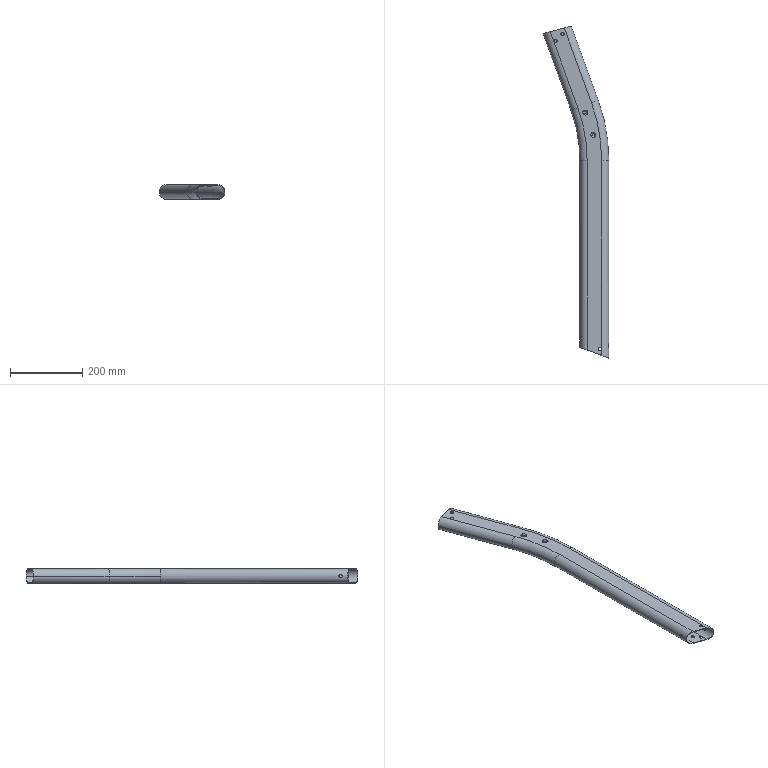Part | STEP file | 5090201R | 1 solid | 43 faces | box 181.681 x 917.444 x 40 mm | volume 273224 mm3 | cylinder 23 | torus 12 | plane 8 | commonest cylinder face diameters 9 x6 37 x6 40 x6 8 x2 11 x2 18 x1